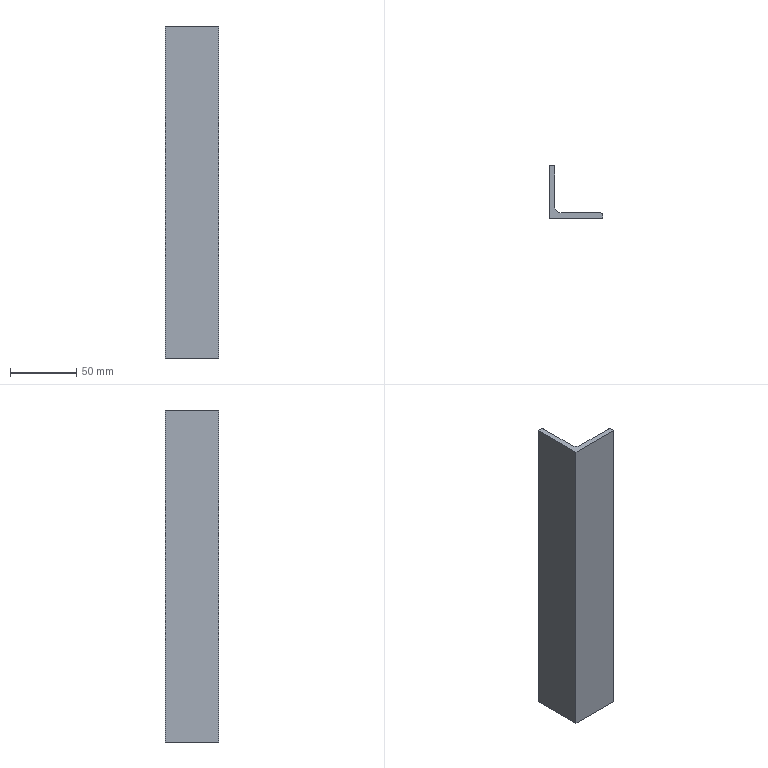Part | SolidWorks | features ICE 1, LibraryFeature 1 | 1 solid | 11 faces | box 40 x 40 x 250 mm | volume 77151 mm3 | plane 8 | cylinder 3 | commonest cylinder face diameters 2.667 x2 10 x1
STEP:
#1=CARTESIAN_POINT('',(9.,4.,0.));
#2=VERTEX_POINT('',#1);
#3=CARTESIAN_POINT('',(4.,9.,0.));
#4=VERTEX_POINT('',#3);
#5=CARTESIAN_POINT('',(9.,9.,0.));
#6=DIRECTION('',(0.,0.,-1.));
#7=DIRECTION('',(-1.,0.,0.));
#8=AXIS2_PLACEMENT_3D('',#5,#6,#7);
#9=CIRCLE('',#8,5.);
#10=EDGE_CURVE('',#2,#4,#9,.T.);
#11=ORIENTED_EDGE('',*,*,#10,.T.);
#12=CARTESIAN_POINT('',(4.,9.,250.));
#13=VERTEX_POINT('',#12);
#14=CARTESIAN_POINT('',(4.,9.,250.));
#15=DIRECTION('',(0.,0.,-1.));
#16=VECTOR('',#15,1000.);
#17=LINE('',#14,#16);
#18=EDGE_CURVE('',#13,#4,#17,.T.);
#19=ORIENTED_EDGE('',*,*,#18,.F.);
#20=CARTESIAN_POINT('',(9.,4.,250.));
#21=VERTEX_POINT('',#20);
#22=CARTESIAN_POINT('',(9.,9.,250.));
#23=DIRECTION('',(0.,0.,-1.));
#24=DIRECTION('',(-1.,0.,0.));
#25=AXIS2_PLACEMENT_3D('',#22,#23,#24);
#26=CIRCLE('',#25,5.);
#27=EDGE_CURVE('',#21,#13,#26,.T.);
#28=ORIENTED_EDGE('',*,*,#27,.F.);
#29=CARTESIAN_POINT('',(9.,4.,250.));
#30=DIRECTION('',(0.,0.,-1.));
#31=VECTOR('',#30,1000.);
#32=LINE('',#29,#31);
#33=EDGE_CURVE('',#21,#2,#32,.T.);
#34=ORIENTED_EDGE('',*,*,#33,.T.);
#35=EDGE_LOOP('',(#11,#19,#28,#34));
#36=FACE_OUTER_BOUND('',#35,.T.);
#37=CARTESIAN_POINT('',(9.,9.,250.));
#38=DIRECTION('',(0.,0.,-1.));
#39=DIRECTION('',(-1.,0.,0.));
#40=AXIS2_PLACEMENT_3D('',#37,#38,#39);
#41=CYLINDRICAL_SURFACE('',#40,5.);
#42=ADVANCED_FACE('',(#36),#41,.F.);
#43=CARTESIAN_POINT('',(4.,38.667,0.));
#44=VERTEX_POINT('',#43);
#45=CARTESIAN_POINT('',(4.,38.667,0.));
#46=DIRECTION('',(0.,-1.,0.));
#47=VECTOR('',#46,1000.);
#48=LINE('',#45,#47);
#49=EDGE_CURVE('',#44,#4,#48,.T.);
#50=ORIENTED_EDGE('',*,*,#49,.F.);
#51=CARTESIAN_POINT('',(4.,38.667,250.));
#52=VERTEX_POINT('',#51);
#53=CARTESIAN_POINT('',(4.,38.667,250.));
#54=DIRECTION('',(0.,0.,-1.));
#55=VECTOR('',#54,1000.);
#56=LINE('',#53,#55);
#57=EDGE_CURVE('',#52,#44,#56,.T.);
#58=ORIENTED_EDGE('',*,*,#57,.F.);
#59=CARTESIAN_POINT('',(4.,38.667,250.));
#60=DIRECTION('',(0.,-1.,0.));
#61=VECTOR('',#60,1000.);
#62=LINE('',#59,#61);
#63=EDGE_CURVE('',#52,#13,#62,.T.);
#64=ORIENTED_EDGE('',*,*,#63,.T.);
#65=ORIENTED_EDGE('',*,*,#18,.T.);
#66=EDGE_LOOP('',(#50,#58,#64,#65));
#67=FACE_OUTER_BOUND('',#66,.T.);
#68=CARTESIAN_POINT('',(4.,38.667,250.));
#69=DIRECTION('',(1.,0.,0.));
#70=DIRECTION('',(0.,1.,0.));
#71=AXIS2_PLACEMENT_3D('',#68,#69,#70);
#72=PLANE('',#71);
#73=ADVANCED_FACE('',(#67),#72,.T.);
#74=CARTESIAN_POINT('',(2.667,40.,0.));
#75=VERTEX_POINT('',#74);
#76=CARTESIAN_POINT('',(2.667,38.667,0.));
#77=DIRECTION('',(0.,0.,-1.));
#78=DIRECTION('',(-1.,0.,0.));
#79=AXIS2_PLACEMENT_3D('',#76,#77,#78);
#80=CIRCLE('',#79,1.333);
#81=EDGE_CURVE('',#75,#44,#80,.T.);
#82=ORIENTED_EDGE('',*,*,#81,.F.);
#83=CARTESIAN_POINT('',(2.667,40.,250.));
#84=VERTEX_POINT('',#83);
#85=CARTESIAN_POINT('',(2.667,40.,250.));
#86=DIRECTION('',(0.,0.,-1.));
#87=VECTOR('',#86,1000.);
#88=LINE('',#85,#87);
#89=EDGE_CURVE('',#84,#75,#88,.T.);
#90=ORIENTED_EDGE('',*,*,#89,.F.);
#91=CARTESIAN_POINT('',(2.667,38.667,250.));
#92=DIRECTION('',(0.,0.,-1.));
#93=DIRECTION('',(-1.,0.,0.));
#94=AXIS2_PLACEMENT_3D('',#91,#92,#93);
#95=CIRCLE('',#94,1.333);
#96=EDGE_CURVE('',#84,#52,#95,.T.);
#97=ORIENTED_EDGE('',*,*,#96,.T.);
#98=ORIENTED_EDGE('',*,*,#57,.T.);
#99=EDGE_LOOP('',(#82,#90,#97,#98));
#100=FACE_OUTER_BOUND('',#99,.T.);
#101=CARTESIAN_POINT('',(2.667,38.667,250.));
#102=DIRECTION('',(0.,0.,-1.));
#103=DIRECTION('',(-1.,0.,0.));
#104=AXIS2_PLACEMENT_3D('',#101,#102,#103);
#105=CYLINDRICAL_SURFACE('',#104,1.333);
#106=ADVANCED_FACE('',(#100),#105,.T.);
#107=CARTESIAN_POINT('',(0.,40.,0.));
#108=VERTEX_POINT('',#107);
#109=CARTESIAN_POINT('',(0.,40.,0.));
#110=DIRECTION('',(1.,0.,0.));
#111=VECTOR('',#110,1000.);
#112=LINE('',#109,#111);
#113=EDGE_CURVE('',#108,#75,#112,.T.);
#114=ORIENTED_EDGE('',*,*,#113,.F.);
#115=CARTESIAN_POINT('',(0.,40.,250.));
#116=VERTEX_POINT('',#115);
#117=CARTESIAN_POINT('',(0.,40.,250.));
#118=DIRECTION('',(0.,0.,-1.));
#119=VECTOR('',#118,1000.);
#120=LINE('',#117,#119);
#121=EDGE_CURVE('',#116,#108,#120,.T.);
#122=ORIENTED_EDGE('',*,*,#121,.F.);
#123=CARTESIAN_POINT('',(0.,40.,250.));
#124=DIRECTION('',(1.,0.,0.));
#125=VECTOR('',#124,1000.);
#126=LINE('',#123,#125);
#127=EDGE_CURVE('',#116,#84,#126,.T.);
#128=ORIENTED_EDGE('',*,*,#127,.T.);
#129=ORIENTED_EDGE('',*,*,#89,.T.);
#130=EDGE_LOOP('',(#114,#122,#128,#129));
#131=FACE_OUTER_BOUND('',#130,.T.);
#132=CARTESIAN_POINT('',(0.,40.,250.));
#133=DIRECTION('',(0.,1.,0.));
#134=DIRECTION('',(0.,0.,1.));
#135=AXIS2_PLACEMENT_3D('',#132,#133,#134);
#136=PLANE('',#135);
#137=ADVANCED_FACE('',(#131),#136,.T.);
#138=CARTESIAN_POINT('',(0.,0.,0.));
#139=VERTEX_POINT('',#138);
#140=CARTESIAN_POINT('',(0.,0.,0.));
#141=DIRECTION('',(0.,1.,0.));
#142=VECTOR('',#141,1000.);
#143=LINE('',#140,#142);
#144=EDGE_CURVE('',#139,#108,#143,.T.);
#145=ORIENTED_EDGE('',*,*,#144,.F.);
#146=CARTESIAN_POINT('',(0.,0.,250.));
#147=VERTEX_POINT('',#146);
#148=CARTESIAN_POINT('',(0.,0.,250.));
#149=DIRECTION('',(0.,0.,-1.));
#150=VECTOR('',#149,1000.);
#151=LINE('',#148,#150);
#152=EDGE_CURVE('',#147,#139,#151,.T.);
#153=ORIENTED_EDGE('',*,*,#152,.F.);
#154=CARTESIAN_POINT('',(0.,0.,250.));
#155=DIRECTION('',(0.,1.,0.));
#156=VECTOR('',#155,1000.);
#157=LINE('',#154,#156);
#158=EDGE_CURVE('',#147,#116,#157,.T.);
#159=ORIENTED_EDGE('',*,*,#158,.T.);
#160=ORIENTED_EDGE('',*,*,#121,.T.);
#161=EDGE_LOOP('',(#145,#153,#159,#160));
#162=FACE_OUTER_BOUND('',#161,.T.);
#163=CARTESIAN_POINT('',(0.,0.,250.));
#164=DIRECTION('',(-1.,0.,0.));
#165=DIRECTION('',(0.,0.,1.));
#166=AXIS2_PLACEMENT_3D('',#163,#164,#165);
#167=PLANE('',#166);
#168=ADVANCED_FACE('',(#162),#167,.T.);
#169=CARTESIAN_POINT('',(40.,0.,0.));
#170=VERTEX_POINT('',#169);
#171=CARTESIAN_POINT('',(40.,0.,0.));
#172=DIRECTION('',(-1.,0.,0.));
#173=VECTOR('',#172,1000.);
#174=LINE('',#171,#173);
#175=EDGE_CURVE('',#170,#139,#174,.T.);
#176=ORIENTED_EDGE('',*,*,#175,.F.);
#177=CARTESIAN_POINT('',(40.,0.,250.));
#178=VERTEX_POINT('',#177);
#179=CARTESIAN_POINT('',(40.,0.,250.));
#180=DIRECTION('',(0.,0.,-1.));
#181=VECTOR('',#180,1000.);
#182=LINE('',#179,#181);
#183=EDGE_CURVE('',#178,#170,#182,.T.);
#184=ORIENTED_EDGE('',*,*,#183,.F.);
#185=CARTESIAN_POINT('',(40.,0.,250.));
#186=DIRECTION('',(-1.,0.,0.));
#187=VECTOR('',#186,1000.);
#188=LINE('',#185,#187);
#189=EDGE_CURVE('',#178,#147,#188,.T.);
#190=ORIENTED_EDGE('',*,*,#189,.T.);
#191=ORIENTED_EDGE('',*,*,#152,.T.);
#192=EDGE_LOOP('',(#176,#184,#190,#191));
#193=FACE_OUTER_BOUND('',#192,.T.);
#194=CARTESIAN_POINT('',(40.,0.,250.));
#195=DIRECTION('',(0.,-1.,0.));
#196=DIRECTION('',(0.,0.,-1.));
#197=AXIS2_PLACEMENT_3D('',#194,#195,#196);
#198=PLANE('',#197);
#199=ADVANCED_FACE('',(#193),#198,.T.);
#200=CARTESIAN_POINT('',(40.,2.667,0.));
#201=VERTEX_POINT('',#200);
#202=CARTESIAN_POINT('',(40.,0.,0.));
#203=DIRECTION('',(0.,1.,0.));
#204=VECTOR('',#203,1000.);
#205=LINE('',#202,#204);
#206=EDGE_CURVE('',#170,#201,#205,.T.);
#207=ORIENTED_EDGE('',*,*,#206,.T.);
#208=CARTESIAN_POINT('',(40.,2.667,250.));
#209=VERTEX_POINT('',#208);
#210=CARTESIAN_POINT('',(40.,2.667,250.));
#211=DIRECTION('',(0.,0.,-1.));
#212=VECTOR('',#211,1000.);
#213=LINE('',#210,#212);
#214=EDGE_CURVE('',#209,#201,#213,.T.);
#215=ORIENTED_EDGE('',*,*,#214,.F.);
#216=CARTESIAN_POINT('',(40.,0.,250.));
#217=DIRECTION('',(0.,1.,0.));
#218=VECTOR('',#217,1000.);
#219=LINE('',#216,#218);
#220=EDGE_CURVE('',#178,#209,#219,.T.);
#221=ORIENTED_EDGE('',*,*,#220,.F.);
#222=ORIENTED_EDGE('',*,*,#183,.T.);
#223=EDGE_LOOP('',(#207,#215,#221,#222));
#224=FACE_OUTER_BOUND('',#223,.T.);
#225=CARTESIAN_POINT('',(40.,0.,250.));
#226=DIRECTION('',(-1.,0.,0.));
#227=DIRECTION('',(0.,0.,1.));
#228=AXIS2_PLACEMENT_3D('',#225,#226,#227);
#229=PLANE('',#228);
#230=ADVANCED_FACE('',(#224),#229,.F.);
#231=CARTESIAN_POINT('',(38.667,4.,0.));
#232=VERTEX_POINT('',#231);
#233=CARTESIAN_POINT('',(38.667,2.667,0.));
#234=DIRECTION('',(0.,0.,1.));
#235=DIRECTION('',(1.,0.,0.));
#236=AXIS2_PLACEMENT_3D('',#233,#234,#235);
#237=CIRCLE('',#236,1.333);
#238=EDGE_CURVE('',#201,#232,#237,.T.);
#239=ORIENTED_EDGE('',*,*,#238,.T.);
#240=CARTESIAN_POINT('',(38.667,4.,250.));
#241=VERTEX_POINT('',#240);
#242=CARTESIAN_POINT('',(38.667,4.,250.));
#243=DIRECTION('',(0.,0.,-1.));
#244=VECTOR('',#243,1000.);
#245=LINE('',#242,#244);
#246=EDGE_CURVE('',#241,#232,#245,.T.);
#247=ORIENTED_EDGE('',*,*,#246,.F.);
#248=CARTESIAN_POINT('',(38.667,2.667,250.));
#249=DIRECTION('',(0.,0.,1.));
#250=DIRECTION('',(1.,0.,0.));
#251=AXIS2_PLACEMENT_3D('',#248,#249,#250);
#252=CIRCLE('',#251,1.333);
#253=EDGE_CURVE('',#209,#241,#252,.T.);
#254=ORIENTED_EDGE('',*,*,#253,.F.);
#255=ORIENTED_EDGE('',*,*,#214,.T.);
#256=EDGE_LOOP('',(#239,#247,#254,#255));
#257=FACE_OUTER_BOUND('',#256,.T.);
#258=CARTESIAN_POINT('',(38.667,2.667,250.));
#259=DIRECTION('',(0.,0.,-1.));
#260=DIRECTION('',(-1.,0.,0.));
#261=AXIS2_PLACEMENT_3D('',#258,#259,#260);
#262=CYLINDRICAL_SURFACE('',#261,1.333);
#263=ADVANCED_FACE('',(#257),#262,.T.);
#264=CARTESIAN_POINT('',(9.,4.,0.));
#265=DIRECTION('',(1.,0.,0.));
#266=VECTOR('',#265,1000.);
#267=LINE('',#264,#266);
#268=EDGE_CURVE('',#2,#232,#267,.T.);
#269=ORIENTED_EDGE('',*,*,#268,.F.);
#270=ORIENTED_EDGE('',*,*,#33,.F.);
#271=CARTESIAN_POINT('',(9.,4.,250.));
#272=DIRECTION('',(1.,0.,0.));
#273=VECTOR('',#272,1000.);
#274=LINE('',#271,#273);
#275=EDGE_CURVE('',#21,#241,#274,.T.);
#276=ORIENTED_EDGE('',*,*,#275,.T.);
#277=ORIENTED_EDGE('',*,*,#246,.T.);
#278=EDGE_LOOP('',(#269,#270,#276,#277));
#279=FACE_OUTER_BOUND('',#278,.T.);
#280=CARTESIAN_POINT('',(9.,4.,250.));
#281=DIRECTION('',(0.,1.,0.));
#282=DIRECTION('',(0.,0.,1.));
#283=AXIS2_PLACEMENT_3D('',#280,#281,#282);
#284=PLANE('',#283);
#285=ADVANCED_FACE('',(#279),#284,.T.);
#286=ORIENTED_EDGE('',*,*,#27,.T.);
#287=ORIENTED_EDGE('',*,*,#63,.F.);
#288=ORIENTED_EDGE('',*,*,#96,.F.);
#289=ORIENTED_EDGE('',*,*,#127,.F.);
#290=ORIENTED_EDGE('',*,*,#158,.F.);
#291=ORIENTED_EDGE('',*,*,#189,.F.);
#292=ORIENTED_EDGE('',*,*,#220,.T.);
#293=ORIENTED_EDGE('',*,*,#253,.T.);
#294=ORIENTED_EDGE('',*,*,#275,.F.);
#295=EDGE_LOOP('',(#286,#287,#288,#289,#290,#291,#292,#293,#294));
#296=FACE_OUTER_BOUND('',#295,.T.);
#297=CARTESIAN_POINT('',(9.,9.,250.));
#298=DIRECTION('',(0.,0.,-1.));
#299=DIRECTION('',(-1.,0.,0.));
#300=AXIS2_PLACEMENT_3D('',#297,#298,#299);
#301=PLANE('',#300);
#302=ADVANCED_FACE('',(#296),#301,.F.);
#303=ORIENTED_EDGE('',*,*,#10,.F.);
#304=ORIENTED_EDGE('',*,*,#268,.T.);
#305=ORIENTED_EDGE('',*,*,#238,.F.);
#306=ORIENTED_EDGE('',*,*,#206,.F.);
#307=ORIENTED_EDGE('',*,*,#175,.T.);
#308=ORIENTED_EDGE('',*,*,#144,.T.);
#309=ORIENTED_EDGE('',*,*,#113,.T.);
#310=ORIENTED_EDGE('',*,*,#81,.T.);
#311=ORIENTED_EDGE('',*,*,#49,.T.);
#312=EDGE_LOOP('',(#303,#304,#305,#306,#307,#308,#309,#310,#311));
#313=FACE_OUTER_BOUND('',#312,.T.);
#314=CARTESIAN_POINT('',(9.,9.,0.));
#315=DIRECTION('',(0.,0.,-1.));
#316=DIRECTION('',(-1.,0.,0.));
#317=AXIS2_PLACEMENT_3D('',#314,#315,#316);
#318=PLANE('',#317);
#319=ADVANCED_FACE('',(#313),#318,.T.);
#320=CLOSED_SHELL('',(#42,#73,#106,#137,#168,#199,#230,#263,#285,#302,#319));
#321=MANIFOLD_SOLID_BREP('',#320);
#322=CARTESIAN_POINT('',(0.,0.,0.));
#323=DIRECTION('',(0.,0.,1.));
#324=DIRECTION('',(1.,0.,0.));
#325=AXIS2_PLACEMENT_3D('',#322,#323,#324);
#326=(LENGTH_UNIT()NAMED_UNIT(*)SI_UNIT(.MILLI.,.METRE.));
#327=UNCERTAINTY_MEASURE_WITH_UNIT(LENGTH_MEASURE(0.00001),#326,'','');
#328=(NAMED_UNIT(*)PLANE_ANGLE_UNIT()SI_UNIT($,.RADIAN.));
#329=(NAMED_UNIT(*)SI_UNIT($,.STERADIAN.)SOLID_ANGLE_UNIT());
#330=(GEOMETRIC_REPRESENTATION_CONTEXT(3)GLOBAL_UNCERTAINTY_ASSIGNED_CONTEXT((#327))GLOBAL_UNIT_ASSIGNED_CONTEXT((#326,#328,#329))REPRESENTATION_CONTEXT('',''));
#331=ADVANCED_BREP_SHAPE_REPRESENTATION('',(#321,#325),#330);